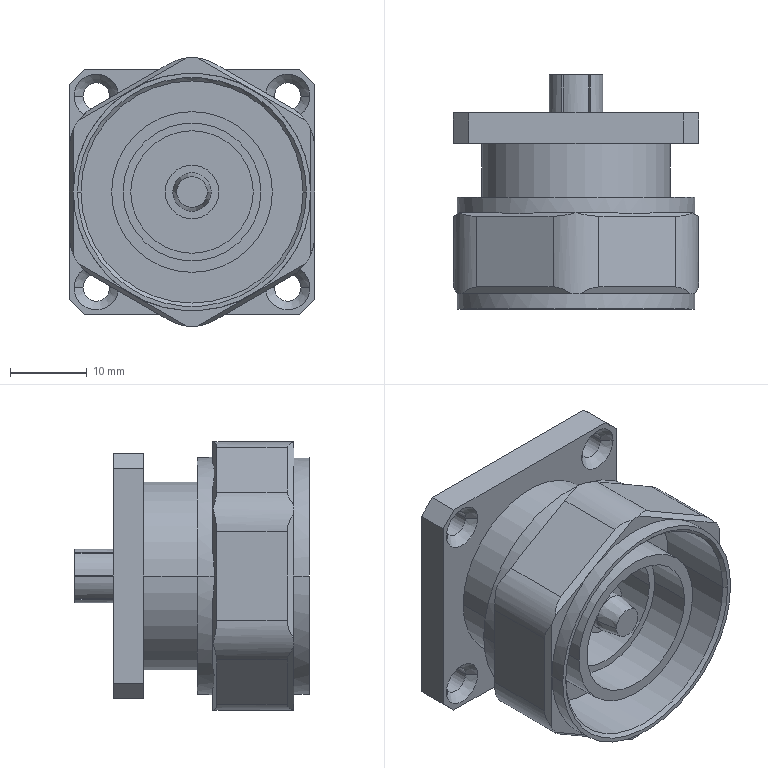Part | STEP file | Connector L29-50JFDA | 3 solids | 143 faces | box 32 x 30.6 x 35.094 mm | volume 12023 mm3 | plane 77 | cylinder 46 | cone 20 | commonest cylinder face diameters 3.5 x8 5 x8 12 x6 7 x4 16 x4 24.6 x4